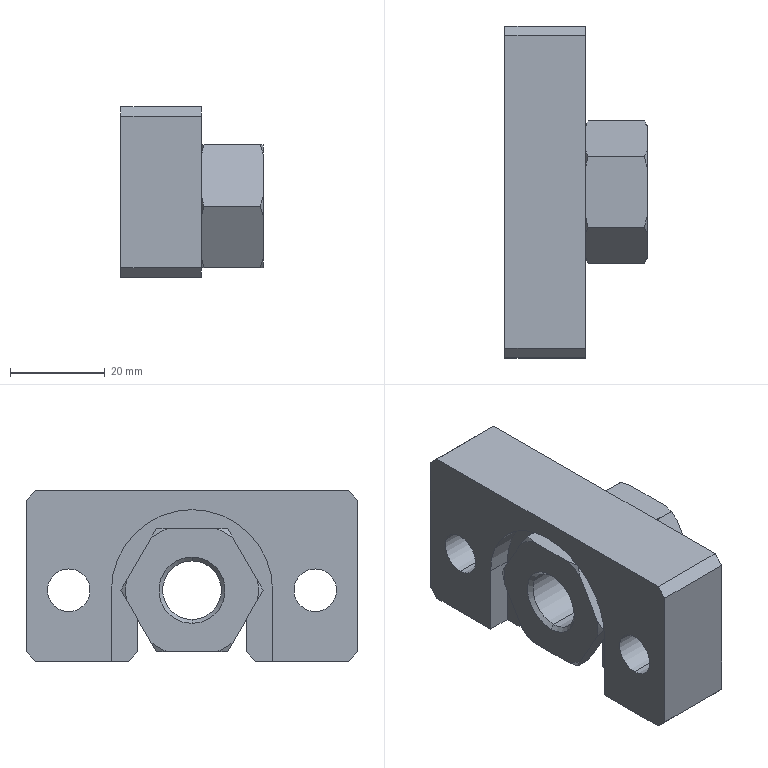Part | STEP file | 001-009-WHD51-M14-1.5 | 2 solids | 91 faces | box 30 x 70 x 36 mm | volume 38071 mm3 | plane 36 | cone 28 | cylinder 27 | commonest cylinder face diameters 30 x12 9 x4 14 x4 12.376 x2 21 x2 23 x2